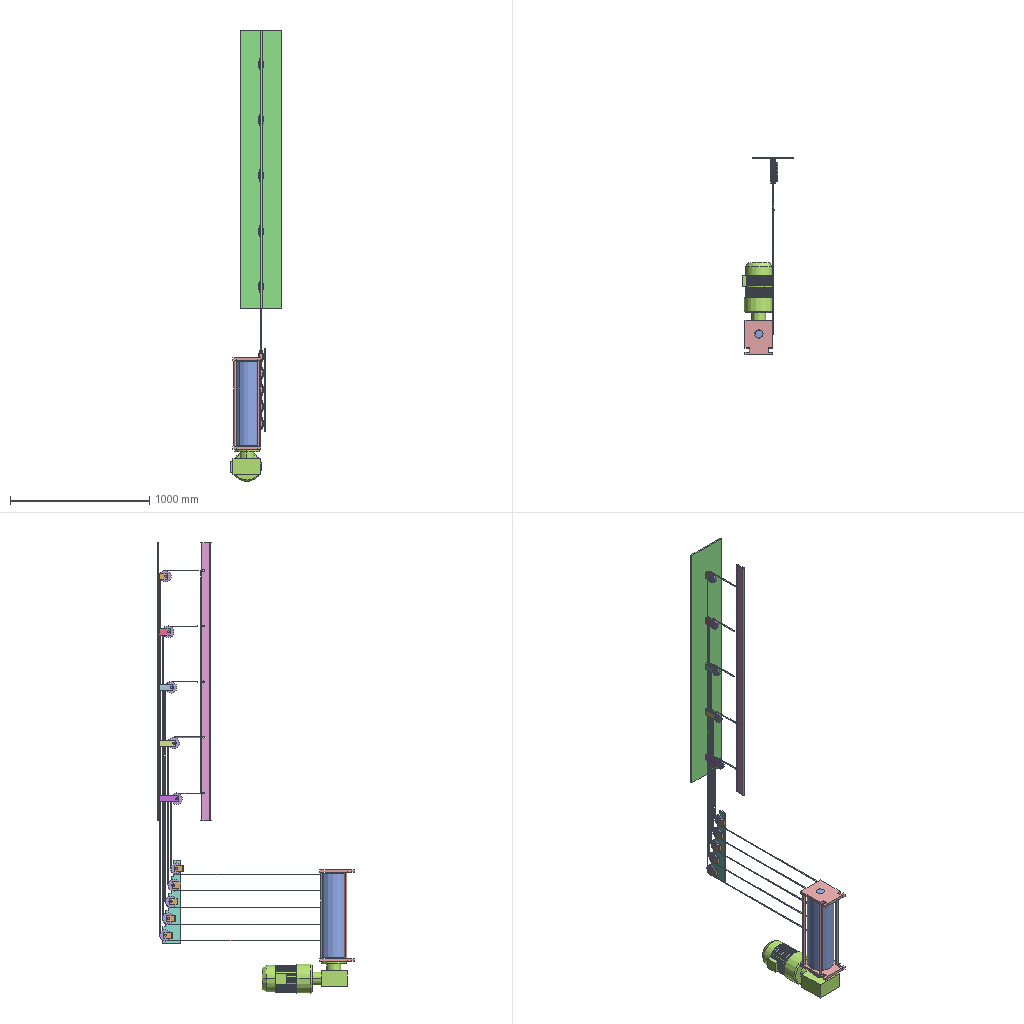Assembly | SolidWorks | 20 different items | 39 placed | box 371 x 1418 x 3239 mm
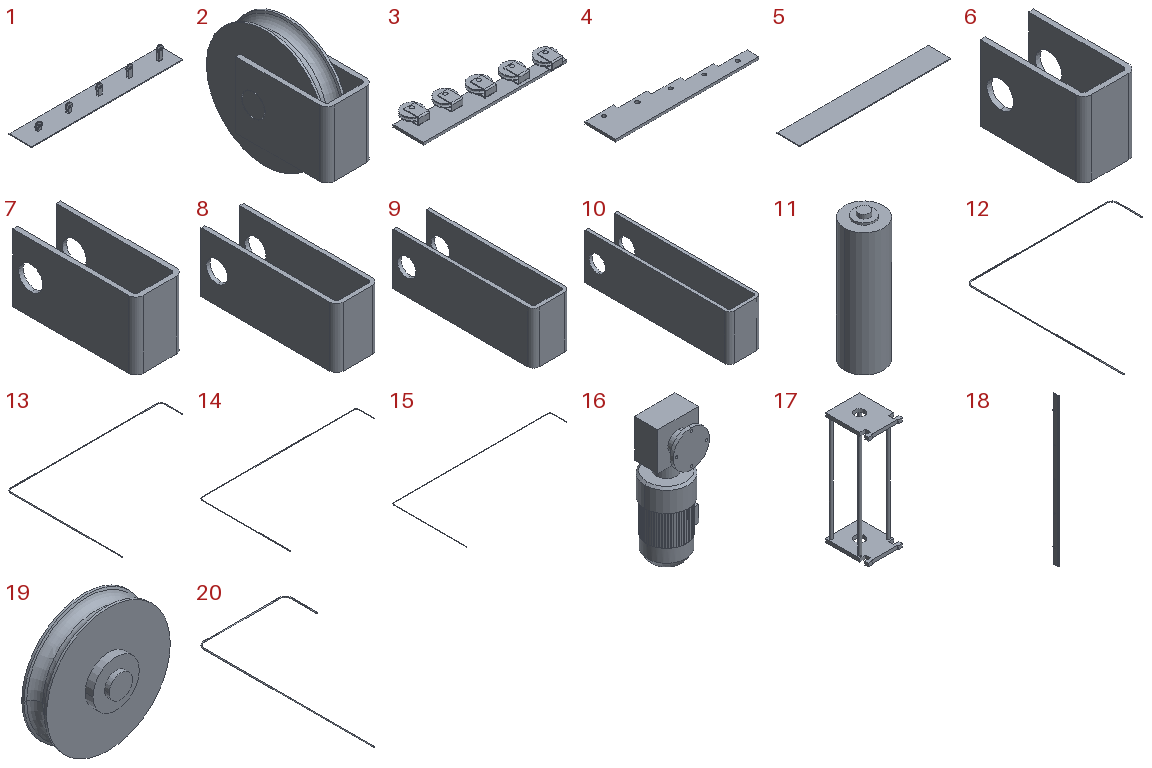Parts list (item | name | quantity | parent item | size | volume | features):
1 | (subassembly) | x1 | - | 2000 x 300 x 180 mm | 6526546 mm3 | -
2 | (subassembly) | x6 | in 1, 3 | 32 x 90 x 80 mm | 94509 mm3 | -
3 | (subassembly) | x1 | - | 600 x 170 x 52 mm | 1003125 mm3 | -
4 | - | x1 | in 3 | 600 x 130 x 10 mm | 530579 mm3 | features Extrusion 1
5 | - | x1 | in 1 | 2000 x 300 x 10 mm | 6000000 mm3 | features Extrusion 1
6 | - | x6 | in 2 | 32 x 62 x 45 mm | 18638 mm3 | features Extrusion 1, ICE 1
7 | - | x1 | in 1 | 32 x 82 x 45 mm | 24038 mm3 | features Extrusion 1, ICE 1
8 | - | x1 | in 1 | 32 x 102 x 45 mm | 29438 mm3 | features Extrusion 1, ICE 1
9 | - | x1 | in 1 | 32 x 122 x 45 mm | 34838 mm3 | features Extrusion 1, ICE 1
10 | - | x1 | in 1 | 32 x 142 x 45 mm | 40238 mm3 | features Extrusion 1, ICE 1
11 | - | x1 | - | 190 x 190 x 660 mm | 17263837 mm3 | features ICE 4, Extrusion 1
12 | - | x1 | - | 1109 x 1198 x 6.5 mm | 82657 mm3 | features Sweep 1
13 | - | x1 | - | 1629 x 1218 x 6.5 mm | 100576 mm3 | features Sweep 1
14 | - | x1 | - | 2149 x 1238 x 6.5 mm | 119159 mm3 | features Sweep 1
15 | - | x1 | - | 2669 x 1258 x 6.5 mm | 138073 mm3 | features Sweep 1
16 | - | x1 | - | 226.9 x 230.198 x 613 mm | 16882473 mm3 | features ICE 11, Chamfer 2, CirPattern 1, Extrusion 1
17 | - | x1 | - | 200 x 250 x 660 mm | 2278181 mm3 | features ICE 2, Extrusion 1
18 | - | x1 | - | 12 x 81 x 2000 mm | 931360 mm3 | features ICE 2, Extrusion 1
19 | - | x10 | in 1, 2 | 80 x 32 x 80 mm | 75871 mm3 | features Revolution 1
20 | - | x1 | - | 588.5 x 1178 x 6.5 mm | 64106 mm3 | features Sweep 1
Mates (type | each side: item.copy, entity, surface, feature):
In the top assembly
Concentric | 17.1 face cylinder Boss-Extrude3 | 11.1 face cylinder Boss-Extrude5
Coincident | 17.1 face plane Boss-Extrude3 | 11.1 face plane Boss-Extrude2
Concentric | 11.1 face cylinder Boss-Extrude1 | 16.1 face cylinder Boss-Extrude10
Coincident | 17.1 face plane Boss-Extrude1 | 16.1 face plane Boss-Extrude11
Parallel | 17.1 face plane Boss-Extrude1 | 16.1 face plane Boss-Extrude3
DistanceDim | 4.1 face plane Boss-Extrude1 | 17.1 face plane Boss-Extrude3
Coincident | 6.1 face plane Boss-Extrude1 | 6.2 face plane Boss-Extrude1
DistanceDim | 10.1 face plane Boss-Extrude1 | 6.1 face plane Boss-Extrude1
DistanceDim | 6.1 face plane Boss-Extrude1 | 10.1 face plane Boss-Extrude1
DistanceDim | 4.1 face plane Boss-Extrude1 | 16.1 face plane Boss-Extrude9 | 2 times
Coincident | 18.1 face plane Boss-Extrude1 | 5.1 face plane Boss-Extrude1
DistanceDim | 18.1 face plane Boss-Extrude1 | 5.1 face plane Boss-Extrude1
DistanceDim | 20.1 face plane Sweep1 | 17.1 face plane Boss-Extrude3
DistanceDim | 20.1 plane | 19.1 face plane Revolve1
Coincident | 20.1 face plane Sweep1 | 12.1 face plane Sweep1
DistanceDim | 12.1 plane | 19.2 face plane Revolve1
Coincident | 12.1 face plane Sweep1 | 13.1 face plane Sweep1
DistanceDim | 13.1 plane | 19.3 face plane Revolve1
Coincident | 20.1 face plane Sweep1 | 14.1 face plane Sweep1
DistanceDim | 14.1 plane | 19.4 face plane Revolve1
Coincident | 20.1 face plane Sweep1 | 15.1 face plane Sweep1
DistanceDim | 15.1 plane | 19.5 face plane Revolve1
In subassembly 3
Concentric | 4.2 face cylinder Boss-Extrude1 | 19.6 face cylinder Revolve1
DistanceDim | 6.3 face plane Boss-Extrude1 | 4.2 face plane Boss-Extrude1
Coincident | 6.3 face plane Boss-Extrude1 | 6.4 face plane Boss-Extrude1
Concentric | 4.2 face cylinder Boss-Extrude1 | 19.7 face cylinder Revolve1
Parallel | 4.2 face plane Boss-Extrude1 | 6.4 face plane Boss-Extrude1
Parallel | 4.2 face plane Boss-Extrude1 | 6.3 face plane Boss-Extrude1
Coincident | 6.4 face plane Boss-Extrude1 | 6.5 face plane Boss-Extrude1
Concentric | 4.2 face cylinder Boss-Extrude1 | 19.8 face cylinder Revolve1
Parallel | 4.2 face plane Boss-Extrude1 | 6.5 face plane Boss-Extrude1
Coincident | 6.5 face plane Boss-Extrude1 | 6.6 face plane Boss-Extrude1
Concentric | 4.2 face cylinder Boss-Extrude1 | 19.9 face cylinder Revolve1
Coincident | 4.2 face plane Boss-Extrude1 | 6.6 face plane Boss-Extrude1
Coincident | 6.6 face plane Boss-Extrude1 | 6.7 face plane Boss-Extrude1
Concentric | 4.2 face cylinder Boss-Extrude1 | 19.10 face cylinder Revolve1
Parallel | 4.2 face plane Boss-Extrude1 | 6.7 face plane Boss-Extrude1
In subassembly 2
Concentric | 6.8 face cylinder Cut-Extrude1 | 19.11 face cylinder Revolve1
Coincident | 6.8 face plane Boss-Extrude1 | 19.11 face plane Revolve1
In subassembly 1
Coincident | 5.2 face plane Boss-Extrude1 | 6.3 face plane Boss-Extrude1
DistanceDim | 6.3 face plane Boss-Extrude1 | 5.2 face plane Boss-Extrude1 | 2 times
Coincident | 5.2 face plane Boss-Extrude1 | 7.1 face plane Boss-Extrude1
Coincident | 6.3 face plane Boss-Extrude1 | 7.1 face plane Boss-Extrude1
DistanceDim | 7.1 face plane Boss-Extrude1 | 6.3 face plane Boss-Extrude1
Coincident | 5.2 face plane Boss-Extrude1 | 8.1 face plane Boss-Extrude1
Coincident | 7.1 face plane Boss-Extrude1 | 8.1 face plane Boss-Extrude1
DistanceDim | 8.1 face plane Boss-Extrude1 | 7.1 face plane Boss-Extrude1
Coincident | 5.2 face plane Boss-Extrude1 | 9.1 face plane Boss-Extrude1
Coincident | 8.1 face plane Boss-Extrude1 | 9.1 face plane Boss-Extrude1
DistanceDim | 9.1 face plane Boss-Extrude1 | 8.1 face plane Boss-Extrude1
Coincident | 5.2 face plane Boss-Extrude1 | 10.2 face plane Boss-Extrude1
Coincident | 9.1 face plane Boss-Extrude1 | 10.2 face plane Boss-Extrude1
DistanceDim | 10.2 face plane Boss-Extrude1 | 9.1 face plane Boss-Extrude1
Concentric | 7.1 face cylinder Cut-Extrude1 | 19.12 face cylinder Revolve1
Coincident | 19.6 face plane Revolve1 | 19.12 face plane Revolve1
Concentric | 8.1 face cylinder Cut-Extrude1 | 19.13 face cylinder Revolve1
Coincident | 19.12 face plane Revolve1 | 19.13 face plane Revolve1
Concentric | 9.1 face cylinder Cut-Extrude1 | 19.14 face cylinder Revolve1
Coincident | 19.13 face plane Revolve1 | 19.14 face plane Revolve1
Concentric | 10.2 face cylinder Cut-Extrude1 | 19.15 face cylinder Revolve1
Coincident | 19.14 face plane Revolve1 | 19.15 face plane Revolve1